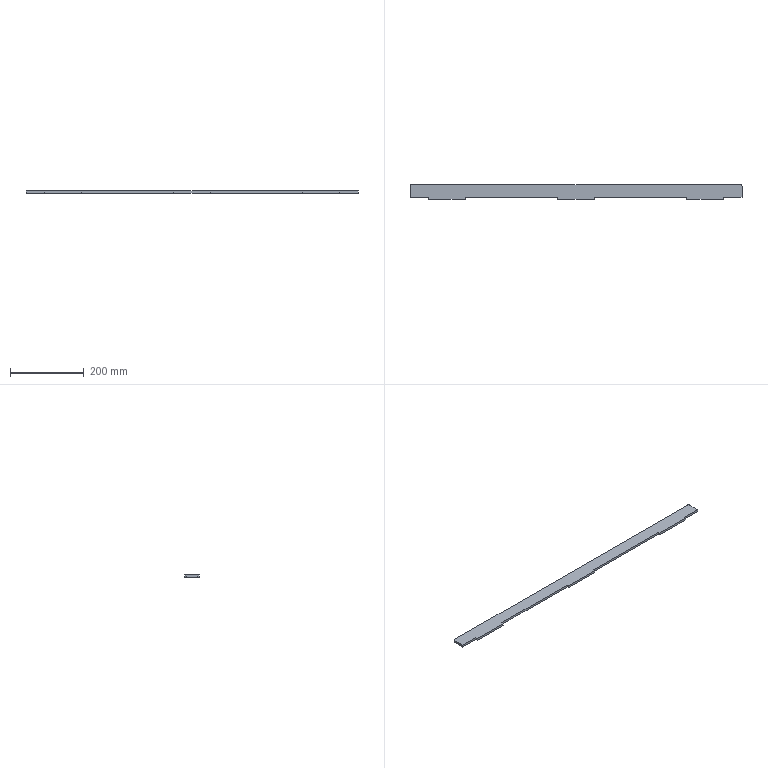Part | SolidWorks | features FlatPattern 1, SMBaseFlange 1, SheetMetal 1 | 1 solid | 20 faces | box 900 x 40.5 x 6 mm | volume 198836 mm3 | plane 18 | cylinder 2 | commonest cylinder face diameters 10 x2
STEP:
#1=CARTESIAN_POINT('',(439.219,-825.02,0.));
#2=VERTEX_POINT('',#1);
#3=CARTESIAN_POINT('',(489.219,-825.02,0.));
#4=VERTEX_POINT('',#3);
#5=CARTESIAN_POINT('',(489.219,-825.02,0.));
#6=DIRECTION('',(1.,0.,0.));
#7=VECTOR('',#6,1000.);
#8=LINE('',#5,#7);
#9=EDGE_CURVE('',#2,#4,#8,.T.);
#10=ORIENTED_EDGE('',*,*,#9,.T.);
#11=CARTESIAN_POINT('',(489.219,-825.02,6.));
#12=VERTEX_POINT('',#11);
#13=CARTESIAN_POINT('',(489.219,-825.02,6.));
#14=DIRECTION('',(0.,0.,-1.));
#15=VECTOR('',#14,1000.);
#16=LINE('',#13,#15);
#17=EDGE_CURVE('',#12,#4,#16,.T.);
#18=ORIENTED_EDGE('',*,*,#17,.F.);
#19=CARTESIAN_POINT('',(439.219,-825.02,6.));
#20=VERTEX_POINT('',#19);
#21=CARTESIAN_POINT('',(489.219,-825.02,6.));
#22=DIRECTION('',(1.,0.,0.));
#23=VECTOR('',#22,1000.);
#24=LINE('',#21,#23);
#25=EDGE_CURVE('',#20,#12,#24,.T.);
#26=ORIENTED_EDGE('',*,*,#25,.F.);
#27=CARTESIAN_POINT('',(439.219,-825.02,6.));
#28=DIRECTION('',(0.,0.,-1.));
#29=VECTOR('',#28,1000.);
#30=LINE('',#27,#29);
#31=EDGE_CURVE('',#20,#2,#30,.T.);
#32=ORIENTED_EDGE('',*,*,#31,.T.);
#33=EDGE_LOOP('',(#10,#18,#26,#32));
#34=FACE_OUTER_BOUND('',#33,.T.);
#35=CARTESIAN_POINT('',(489.219,-825.02,6.));
#36=DIRECTION('',(0.,1.,0.));
#37=DIRECTION('',(0.,0.,1.));
#38=AXIS2_PLACEMENT_3D('',#35,#36,#37);
#39=PLANE('',#38);
#40=ADVANCED_FACE('',(#34),#39,.F.);
#41=CARTESIAN_POINT('',(489.219,-795.02,0.));
#42=VERTEX_POINT('',#41);
#43=CARTESIAN_POINT('',(489.219,-825.02,0.));
#44=DIRECTION('',(0.,1.,0.));
#45=VECTOR('',#44,1000.);
#46=LINE('',#43,#45);
#47=EDGE_CURVE('',#4,#42,#46,.T.);
#48=ORIENTED_EDGE('',*,*,#47,.T.);
#49=CARTESIAN_POINT('',(489.219,-795.02,6.));
#50=VERTEX_POINT('',#49);
#51=CARTESIAN_POINT('',(489.219,-795.02,6.));
#52=DIRECTION('',(0.,0.,-1.));
#53=VECTOR('',#52,1000.);
#54=LINE('',#51,#53);
#55=EDGE_CURVE('',#50,#42,#54,.T.);
#56=ORIENTED_EDGE('',*,*,#55,.F.);
#57=CARTESIAN_POINT('',(489.219,-825.02,6.));
#58=DIRECTION('',(0.,1.,0.));
#59=VECTOR('',#58,1000.);
#60=LINE('',#57,#59);
#61=EDGE_CURVE('',#12,#50,#60,.T.);
#62=ORIENTED_EDGE('',*,*,#61,.F.);
#63=ORIENTED_EDGE('',*,*,#17,.T.);
#64=EDGE_LOOP('',(#48,#56,#62,#63));
#65=FACE_OUTER_BOUND('',#64,.T.);
#66=CARTESIAN_POINT('',(489.219,-825.02,6.));
#67=DIRECTION('',(-1.,0.,0.));
#68=DIRECTION('',(0.,0.,1.));
#69=AXIS2_PLACEMENT_3D('',#66,#67,#68);
#70=PLANE('',#69);
#71=ADVANCED_FACE('',(#65),#70,.F.);
#72=CARTESIAN_POINT('',(484.219,-790.02,0.));
#73=VERTEX_POINT('',#72);
#74=CARTESIAN_POINT('',(484.219,-795.02,0.));
#75=DIRECTION('',(0.,0.,1.));
#76=DIRECTION('',(1.,0.,0.));
#77=AXIS2_PLACEMENT_3D('',#74,#75,#76);
#78=CIRCLE('',#77,5.);
#79=EDGE_CURVE('',#42,#73,#78,.T.);
#80=ORIENTED_EDGE('',*,*,#79,.T.);
#81=CARTESIAN_POINT('',(484.219,-790.02,6.));
#82=VERTEX_POINT('',#81);
#83=CARTESIAN_POINT('',(484.219,-790.02,6.));
#84=DIRECTION('',(0.,0.,-1.));
#85=VECTOR('',#84,1000.);
#86=LINE('',#83,#85);
#87=EDGE_CURVE('',#82,#73,#86,.T.);
#88=ORIENTED_EDGE('',*,*,#87,.F.);
#89=CARTESIAN_POINT('',(484.219,-795.02,6.));
#90=DIRECTION('',(0.,0.,1.));
#91=DIRECTION('',(1.,0.,0.));
#92=AXIS2_PLACEMENT_3D('',#89,#90,#91);
#93=CIRCLE('',#92,5.);
#94=EDGE_CURVE('',#50,#82,#93,.T.);
#95=ORIENTED_EDGE('',*,*,#94,.F.);
#96=ORIENTED_EDGE('',*,*,#55,.T.);
#97=EDGE_LOOP('',(#80,#88,#95,#96));
#98=FACE_OUTER_BOUND('',#97,.T.);
#99=CARTESIAN_POINT('',(484.219,-795.02,6.));
#100=DIRECTION('',(0.,0.,-1.));
#101=DIRECTION('',(-1.,0.,0.));
#102=AXIS2_PLACEMENT_3D('',#99,#100,#101);
#103=CYLINDRICAL_SURFACE('',#102,5.);
#104=ADVANCED_FACE('',(#98),#103,.T.);
#105=CARTESIAN_POINT('',(-405.781,-790.02,0.));
#106=VERTEX_POINT('',#105);
#107=CARTESIAN_POINT('',(484.219,-790.02,0.));
#108=DIRECTION('',(-1.,0.,0.));
#109=VECTOR('',#108,1000.);
#110=LINE('',#107,#109);
#111=EDGE_CURVE('',#73,#106,#110,.T.);
#112=ORIENTED_EDGE('',*,*,#111,.T.);
#113=CARTESIAN_POINT('',(-405.781,-790.02,6.));
#114=VERTEX_POINT('',#113);
#115=CARTESIAN_POINT('',(-405.781,-790.02,6.));
#116=DIRECTION('',(0.,0.,-1.));
#117=VECTOR('',#116,1000.);
#118=LINE('',#115,#117);
#119=EDGE_CURVE('',#114,#106,#118,.T.);
#120=ORIENTED_EDGE('',*,*,#119,.F.);
#121=CARTESIAN_POINT('',(484.219,-790.02,6.));
#122=DIRECTION('',(-1.,0.,0.));
#123=VECTOR('',#122,1000.);
#124=LINE('',#121,#123);
#125=EDGE_CURVE('',#82,#114,#124,.T.);
#126=ORIENTED_EDGE('',*,*,#125,.F.);
#127=ORIENTED_EDGE('',*,*,#87,.T.);
#128=EDGE_LOOP('',(#112,#120,#126,#127));
#129=FACE_OUTER_BOUND('',#128,.T.);
#130=CARTESIAN_POINT('',(484.219,-790.02,6.));
#131=DIRECTION('',(0.,-1.,0.));
#132=DIRECTION('',(1.,0.,0.));
#133=AXIS2_PLACEMENT_3D('',#130,#131,#132);
#134=PLANE('',#133);
#135=ADVANCED_FACE('',(#129),#134,.F.);
#136=CARTESIAN_POINT('',(-410.781,-795.02,0.));
#137=VERTEX_POINT('',#136);
#138=CARTESIAN_POINT('',(-405.781,-795.02,0.));
#139=DIRECTION('',(0.,0.,1.));
#140=DIRECTION('',(1.,0.,0.));
#141=AXIS2_PLACEMENT_3D('',#138,#139,#140);
#142=CIRCLE('',#141,5.);
#143=EDGE_CURVE('',#106,#137,#142,.T.);
#144=ORIENTED_EDGE('',*,*,#143,.T.);
#145=CARTESIAN_POINT('',(-410.781,-795.02,6.));
#146=VERTEX_POINT('',#145);
#147=CARTESIAN_POINT('',(-410.781,-795.02,6.));
#148=DIRECTION('',(0.,0.,-1.));
#149=VECTOR('',#148,1000.);
#150=LINE('',#147,#149);
#151=EDGE_CURVE('',#146,#137,#150,.T.);
#152=ORIENTED_EDGE('',*,*,#151,.F.);
#153=CARTESIAN_POINT('',(-405.781,-795.02,6.));
#154=DIRECTION('',(0.,0.,1.));
#155=DIRECTION('',(1.,0.,0.));
#156=AXIS2_PLACEMENT_3D('',#153,#154,#155);
#157=CIRCLE('',#156,5.);
#158=EDGE_CURVE('',#114,#146,#157,.T.);
#159=ORIENTED_EDGE('',*,*,#158,.F.);
#160=ORIENTED_EDGE('',*,*,#119,.T.);
#161=EDGE_LOOP('',(#144,#152,#159,#160));
#162=FACE_OUTER_BOUND('',#161,.T.);
#163=CARTESIAN_POINT('',(-405.781,-795.02,6.));
#164=DIRECTION('',(0.,0.,-1.));
#165=DIRECTION('',(-1.,0.,0.));
#166=AXIS2_PLACEMENT_3D('',#163,#164,#165);
#167=CYLINDRICAL_SURFACE('',#166,5.);
#168=ADVANCED_FACE('',(#162),#167,.T.);
#169=CARTESIAN_POINT('',(-410.781,-825.02,0.));
#170=VERTEX_POINT('',#169);
#171=CARTESIAN_POINT('',(-410.781,-825.02,0.));
#172=DIRECTION('',(0.,-1.,0.));
#173=VECTOR('',#172,1000.);
#174=LINE('',#171,#173);
#175=EDGE_CURVE('',#137,#170,#174,.T.);
#176=ORIENTED_EDGE('',*,*,#175,.T.);
#177=CARTESIAN_POINT('',(-410.781,-825.02,6.));
#178=VERTEX_POINT('',#177);
#179=CARTESIAN_POINT('',(-410.781,-825.02,6.));
#180=DIRECTION('',(0.,0.,-1.));
#181=VECTOR('',#180,1000.);
#182=LINE('',#179,#181);
#183=EDGE_CURVE('',#178,#170,#182,.T.);
#184=ORIENTED_EDGE('',*,*,#183,.F.);
#185=CARTESIAN_POINT('',(-410.781,-825.02,6.));
#186=DIRECTION('',(0.,-1.,0.));
#187=VECTOR('',#186,1000.);
#188=LINE('',#185,#187);
#189=EDGE_CURVE('',#146,#178,#188,.T.);
#190=ORIENTED_EDGE('',*,*,#189,.F.);
#191=ORIENTED_EDGE('',*,*,#151,.T.);
#192=EDGE_LOOP('',(#176,#184,#190,#191));
#193=FACE_OUTER_BOUND('',#192,.T.);
#194=CARTESIAN_POINT('',(-410.781,-825.02,6.));
#195=DIRECTION('',(1.,0.,0.));
#196=DIRECTION('',(0.,1.,0.));
#197=AXIS2_PLACEMENT_3D('',#194,#195,#196);
#198=PLANE('',#197);
#199=ADVANCED_FACE('',(#193),#198,.F.);
#200=CARTESIAN_POINT('',(-360.781,-825.02,0.));
#201=VERTEX_POINT('',#200);
#202=CARTESIAN_POINT('',(-360.781,-825.02,0.));
#203=DIRECTION('',(1.,0.,0.));
#204=VECTOR('',#203,1000.);
#205=LINE('',#202,#204);
#206=EDGE_CURVE('',#170,#201,#205,.T.);
#207=ORIENTED_EDGE('',*,*,#206,.T.);
#208=CARTESIAN_POINT('',(-360.781,-825.02,6.));
#209=VERTEX_POINT('',#208);
#210=CARTESIAN_POINT('',(-360.781,-825.02,6.));
#211=DIRECTION('',(0.,0.,-1.));
#212=VECTOR('',#211,1000.);
#213=LINE('',#210,#212);
#214=EDGE_CURVE('',#209,#201,#213,.T.);
#215=ORIENTED_EDGE('',*,*,#214,.F.);
#216=CARTESIAN_POINT('',(-360.781,-825.02,6.));
#217=DIRECTION('',(1.,0.,0.));
#218=VECTOR('',#217,1000.);
#219=LINE('',#216,#218);
#220=EDGE_CURVE('',#178,#209,#219,.T.);
#221=ORIENTED_EDGE('',*,*,#220,.F.);
#222=ORIENTED_EDGE('',*,*,#183,.T.);
#223=EDGE_LOOP('',(#207,#215,#221,#222));
#224=FACE_OUTER_BOUND('',#223,.T.);
#225=CARTESIAN_POINT('',(-360.781,-825.02,6.));
#226=DIRECTION('',(0.,1.,0.));
#227=DIRECTION('',(-1.,0.,0.));
#228=AXIS2_PLACEMENT_3D('',#225,#226,#227);
#229=PLANE('',#228);
#230=ADVANCED_FACE('',(#224),#229,.F.);
#231=CARTESIAN_POINT('',(-360.781,-830.52,0.));
#232=VERTEX_POINT('',#231);
#233=CARTESIAN_POINT('',(-360.781,-830.52,0.));
#234=DIRECTION('',(0.,-1.,0.));
#235=VECTOR('',#234,1000.);
#236=LINE('',#233,#235);
#237=EDGE_CURVE('',#201,#232,#236,.T.);
#238=ORIENTED_EDGE('',*,*,#237,.T.);
#239=CARTESIAN_POINT('',(-360.781,-830.52,6.));
#240=VERTEX_POINT('',#239);
#241=CARTESIAN_POINT('',(-360.781,-830.52,6.));
#242=DIRECTION('',(0.,0.,-1.));
#243=VECTOR('',#242,1000.);
#244=LINE('',#241,#243);
#245=EDGE_CURVE('',#240,#232,#244,.T.);
#246=ORIENTED_EDGE('',*,*,#245,.F.);
#247=CARTESIAN_POINT('',(-360.781,-830.52,6.));
#248=DIRECTION('',(0.,-1.,0.));
#249=VECTOR('',#248,1000.);
#250=LINE('',#247,#249);
#251=EDGE_CURVE('',#209,#240,#250,.T.);
#252=ORIENTED_EDGE('',*,*,#251,.F.);
#253=ORIENTED_EDGE('',*,*,#214,.T.);
#254=EDGE_LOOP('',(#238,#246,#252,#253));
#255=FACE_OUTER_BOUND('',#254,.T.);
#256=CARTESIAN_POINT('',(-360.781,-830.52,6.));
#257=DIRECTION('',(1.,0.,0.));
#258=DIRECTION('',(0.,0.,-1.));
#259=AXIS2_PLACEMENT_3D('',#256,#257,#258);
#260=PLANE('',#259);
#261=ADVANCED_FACE('',(#255),#260,.F.);
#262=CARTESIAN_POINT('',(-260.781,-830.52,0.));
#263=VERTEX_POINT('',#262);
#264=CARTESIAN_POINT('',(-260.781,-830.52,0.));
#265=DIRECTION('',(1.,0.,0.));
#266=VECTOR('',#265,1000.);
#267=LINE('',#264,#266);
#268=EDGE_CURVE('',#232,#263,#267,.T.);
#269=ORIENTED_EDGE('',*,*,#268,.T.);
#270=CARTESIAN_POINT('',(-260.781,-830.52,6.));
#271=VERTEX_POINT('',#270);
#272=CARTESIAN_POINT('',(-260.781,-830.52,6.));
#273=DIRECTION('',(0.,0.,-1.));
#274=VECTOR('',#273,1000.);
#275=LINE('',#272,#274);
#276=EDGE_CURVE('',#271,#263,#275,.T.);
#277=ORIENTED_EDGE('',*,*,#276,.F.);
#278=CARTESIAN_POINT('',(-260.781,-830.52,6.));
#279=DIRECTION('',(1.,0.,0.));
#280=VECTOR('',#279,1000.);
#281=LINE('',#278,#280);
#282=EDGE_CURVE('',#240,#271,#281,.T.);
#283=ORIENTED_EDGE('',*,*,#282,.F.);
#284=ORIENTED_EDGE('',*,*,#245,.T.);
#285=EDGE_LOOP('',(#269,#277,#283,#284));
#286=FACE_OUTER_BOUND('',#285,.T.);
#287=CARTESIAN_POINT('',(-260.781,-830.52,6.));
#288=DIRECTION('',(0.,1.,0.));
#289=DIRECTION('',(0.,0.,1.));
#290=AXIS2_PLACEMENT_3D('',#287,#288,#289);
#291=PLANE('',#290);
#292=ADVANCED_FACE('',(#286),#291,.F.);
#293=CARTESIAN_POINT('',(-260.781,-825.02,0.));
#294=VERTEX_POINT('',#293);
#295=CARTESIAN_POINT('',(-260.781,-825.02,0.));
#296=DIRECTION('',(0.,1.,0.));
#297=VECTOR('',#296,1000.);
#298=LINE('',#295,#297);
#299=EDGE_CURVE('',#263,#294,#298,.T.);
#300=ORIENTED_EDGE('',*,*,#299,.T.);
#301=CARTESIAN_POINT('',(-260.781,-825.02,6.));
#302=VERTEX_POINT('',#301);
#303=CARTESIAN_POINT('',(-260.781,-825.02,6.));
#304=DIRECTION('',(0.,0.,-1.));
#305=VECTOR('',#304,1000.);
#306=LINE('',#303,#305);
#307=EDGE_CURVE('',#302,#294,#306,.T.);
#308=ORIENTED_EDGE('',*,*,#307,.F.);
#309=CARTESIAN_POINT('',(-260.781,-825.02,6.));
#310=DIRECTION('',(0.,1.,0.));
#311=VECTOR('',#310,1000.);
#312=LINE('',#309,#311);
#313=EDGE_CURVE('',#271,#302,#312,.T.);
#314=ORIENTED_EDGE('',*,*,#313,.F.);
#315=ORIENTED_EDGE('',*,*,#276,.T.);
#316=EDGE_LOOP('',(#300,#308,#314,#315));
#317=FACE_OUTER_BOUND('',#316,.T.);
#318=CARTESIAN_POINT('',(-260.781,-825.02,6.));
#319=DIRECTION('',(-1.,0.,0.));
#320=DIRECTION('',(0.,0.,1.));
#321=AXIS2_PLACEMENT_3D('',#318,#319,#320);
#322=PLANE('',#321);
#323=ADVANCED_FACE('',(#317),#322,.F.);
#324=CARTESIAN_POINT('',(-10.781,-825.02,0.));
#325=VERTEX_POINT('',#324);
#326=CARTESIAN_POINT('',(-10.781,-825.02,0.));
#327=DIRECTION('',(1.,0.,0.));
#328=VECTOR('',#327,1000.);
#329=LINE('',#326,#328);
#330=EDGE_CURVE('',#294,#325,#329,.T.);
#331=ORIENTED_EDGE('',*,*,#330,.T.);
#332=CARTESIAN_POINT('',(-10.781,-825.02,6.));
#333=VERTEX_POINT('',#332);
#334=CARTESIAN_POINT('',(-10.781,-825.02,6.));
#335=DIRECTION('',(0.,0.,-1.));
#336=VECTOR('',#335,1000.);
#337=LINE('',#334,#336);
#338=EDGE_CURVE('',#333,#325,#337,.T.);
#339=ORIENTED_EDGE('',*,*,#338,.F.);
#340=CARTESIAN_POINT('',(-10.781,-825.02,6.));
#341=DIRECTION('',(1.,0.,0.));
#342=VECTOR('',#341,1000.);
#343=LINE('',#340,#342);
#344=EDGE_CURVE('',#302,#333,#343,.T.);
#345=ORIENTED_EDGE('',*,*,#344,.F.);
#346=ORIENTED_EDGE('',*,*,#307,.T.);
#347=EDGE_LOOP('',(#331,#339,#345,#346));
#348=FACE_OUTER_BOUND('',#347,.T.);
#349=CARTESIAN_POINT('',(-10.781,-825.02,6.));
#350=DIRECTION('',(0.,1.,0.));
#351=DIRECTION('',(-1.,0.,0.));
#352=AXIS2_PLACEMENT_3D('',#349,#350,#351);
#353=PLANE('',#352);
#354=ADVANCED_FACE('',(#348),#353,.F.);
#355=CARTESIAN_POINT('',(-10.781,-830.52,0.));
#356=VERTEX_POINT('',#355);
#357=CARTESIAN_POINT('',(-10.781,-830.52,0.));
#358=DIRECTION('',(0.,-1.,0.));
#359=VECTOR('',#358,1000.);
#360=LINE('',#357,#359);
#361=EDGE_CURVE('',#325,#356,#360,.T.);
#362=ORIENTED_EDGE('',*,*,#361,.T.);
#363=CARTESIAN_POINT('',(-10.781,-830.52,6.));
#364=VERTEX_POINT('',#363);
#365=CARTESIAN_POINT('',(-10.781,-830.52,6.));
#366=DIRECTION('',(0.,0.,-1.));
#367=VECTOR('',#366,1000.);
#368=LINE('',#365,#367);
#369=EDGE_CURVE('',#364,#356,#368,.T.);
#370=ORIENTED_EDGE('',*,*,#369,.F.);
#371=CARTESIAN_POINT('',(-10.781,-830.52,6.));
#372=DIRECTION('',(0.,-1.,0.));
#373=VECTOR('',#372,1000.);
#374=LINE('',#371,#373);
#375=EDGE_CURVE('',#333,#364,#374,.T.);
#376=ORIENTED_EDGE('',*,*,#375,.F.);
#377=ORIENTED_EDGE('',*,*,#338,.T.);
#378=EDGE_LOOP('',(#362,#370,#376,#377));
#379=FACE_OUTER_BOUND('',#378,.T.);
#380=CARTESIAN_POINT('',(-10.781,-830.52,6.));
#381=DIRECTION('',(1.,0.,0.));
#382=DIRECTION('',(0.,0.,-1.));
#383=AXIS2_PLACEMENT_3D('',#380,#381,#382);
#384=PLANE('',#383);
#385=ADVANCED_FACE('',(#379),#384,.F.);
#386=CARTESIAN_POINT('',(89.219,-830.52,0.));
#387=VERTEX_POINT('',#386);
#388=CARTESIAN_POINT('',(89.219,-830.52,0.));
#389=DIRECTION('',(1.,0.,0.));
#390=VECTOR('',#389,1000.);
#391=LINE('',#388,#390);
#392=EDGE_CURVE('',#356,#387,#391,.T.);
#393=ORIENTED_EDGE('',*,*,#392,.T.);
#394=CARTESIAN_POINT('',(89.219,-830.52,6.));
#395=VERTEX_POINT('',#394);
#396=CARTESIAN_POINT('',(89.219,-830.52,6.));
#397=DIRECTION('',(0.,0.,-1.));
#398=VECTOR('',#397,1000.);
#399=LINE('',#396,#398);
#400=EDGE_CURVE('',#395,#387,#399,.T.);
#401=ORIENTED_EDGE('',*,*,#400,.F.);
#402=CARTESIAN_POINT('',(89.219,-830.52,6.));
#403=DIRECTION('',(1.,0.,0.));
#404=VECTOR('',#403,1000.);
#405=LINE('',#402,#404);
#406=EDGE_CURVE('',#364,#395,#405,.T.);
#407=ORIENTED_EDGE('',*,*,#406,.F.);
#408=ORIENTED_EDGE('',*,*,#369,.T.);
#409=EDGE_LOOP('',(#393,#401,#407,#408));
#410=FACE_OUTER_BOUND('',#409,.T.);
#411=CARTESIAN_POINT('',(89.219,-830.52,6.));
#412=DIRECTION('',(0.,1.,0.));
#413=DIRECTION('',(0.,0.,1.));
#414=AXIS2_PLACEMENT_3D('',#411,#412,#413);
#415=PLANE('',#414);
#416=ADVANCED_FACE('',(#410),#415,.F.);
#417=CARTESIAN_POINT('',(89.219,-825.02,0.));
#418=VERTEX_POINT('',#417);
#419=CARTESIAN_POINT('',(89.219,-825.02,0.));
#420=DIRECTION('',(0.,1.,0.));
#421=VECTOR('',#420,1000.);
#422=LINE('',#419,#421);
#423=EDGE_CURVE('',#387,#418,#422,.T.);
#424=ORIENTED_EDGE('',*,*,#423,.T.);
#425=CARTESIAN_POINT('',(89.219,-825.02,6.));
#426=VERTEX_POINT('',#425);
#427=CARTESIAN_POINT('',(89.219,-825.02,6.));
#428=DIRECTION('',(0.,0.,-1.));
#429=VECTOR('',#428,1000.);
#430=LINE('',#427,#429);
#431=EDGE_CURVE('',#426,#418,#430,.T.);
#432=ORIENTED_EDGE('',*,*,#431,.F.);
#433=CARTESIAN_POINT('',(89.219,-825.02,6.));
#434=DIRECTION('',(0.,1.,0.));
#435=VECTOR('',#434,1000.);
#436=LINE('',#433,#435);
#437=EDGE_CURVE('',#395,#426,#436,.T.);
#438=ORIENTED_EDGE('',*,*,#437,.F.);
#439=ORIENTED_EDGE('',*,*,#400,.T.);
#440=EDGE_LOOP('',(#424,#432,#438,#439));
#441=FACE_OUTER_BOUND('',#440,.T.);
#442=CARTESIAN_POINT('',(89.219,-825.02,6.));
#443=DIRECTION('',(-1.,0.,0.));
#444=DIRECTION('',(0.,0.,1.));
#445=AXIS2_PLACEMENT_3D('',#442,#443,#444);
#446=PLANE('',#445);
#447=ADVANCED_FACE('',(#441),#446,.F.);
#448=CARTESIAN_POINT('',(339.219,-825.02,0.));
#449=VERTEX_POINT('',#448);
#450=CARTESIAN_POINT('',(339.219,-825.02,0.));
#451=DIRECTION('',(1.,0.,0.));
#452=VECTOR('',#451,1000.);
#453=LINE('',#450,#452);
#454=EDGE_CURVE('',#418,#449,#453,.T.);
#455=ORIENTED_EDGE('',*,*,#454,.T.);
#456=CARTESIAN_POINT('',(339.219,-825.02,6.));
#457=VERTEX_POINT('',#456);
#458=CARTESIAN_POINT('',(339.219,-825.02,6.));
#459=DIRECTION('',(0.,0.,-1.));
#460=VECTOR('',#459,1000.);
#461=LINE('',#458,#460);
#462=EDGE_CURVE('',#457,#449,#461,.T.);
#463=ORIENTED_EDGE('',*,*,#462,.F.);
#464=CARTESIAN_POINT('',(339.219,-825.02,6.));
#465=DIRECTION('',(1.,0.,0.));
#466=VECTOR('',#465,1000.);
#467=LINE('',#464,#466);
#468=EDGE_CURVE('',#426,#457,#467,.T.);
#469=ORIENTED_EDGE('',*,*,#468,.F.);
#470=ORIENTED_EDGE('',*,*,#431,.T.);
#471=EDGE_LOOP('',(#455,#463,#469,#470));
#472=FACE_OUTER_BOUND('',#471,.T.);
#473=CARTESIAN_POINT('',(339.219,-825.02,6.));
#474=DIRECTION('',(0.,1.,0.));
#475=DIRECTION('',(-1.,0.,0.));
#476=AXIS2_PLACEMENT_3D('',#473,#474,#475);
#477=PLANE('',#476);
#478=ADVANCED_FACE('',(#472),#477,.F.);
#479=CARTESIAN_POINT('',(339.219,-830.52,0.));
#480=VERTEX_POINT('',#479);
#481=CARTESIAN_POINT('',(339.219,-830.52,0.));
#482=DIRECTION('',(0.,-1.,0.));
#483=VECTOR('',#482,1000.);
#484=LINE('',#481,#483);
#485=EDGE_CURVE('',#449,#480,#484,.T.);
#486=ORIENTED_EDGE('',*,*,#485,.T.);
#487=CARTESIAN_POINT('',(339.219,-830.52,6.));
#488=VERTEX_POINT('',#487);
#489=CARTESIAN_POINT('',(339.219,-830.52,6.));
#490=DIRECTION('',(0.,0.,-1.));
#491=VECTOR('',#490,1000.);
#492=LINE('',#489,#491);
#493=EDGE_CURVE('',#488,#480,#492,.T.);
#494=ORIENTED_EDGE('',*,*,#493,.F.);
#495=CARTESIAN_POINT('',(339.219,-830.52,6.));
#496=DIRECTION('',(0.,-1.,0.));
#497=VECTOR('',#496,1000.);
#498=LINE('',#495,#497);
#499=EDGE_CURVE('',#457,#488,#498,.T.);
#500=ORIENTED_EDGE('',*,*,#499,.F.);
#501=ORIENTED_EDGE('',*,*,#462,.T.);
#502=EDGE_LOOP('',(#486,#494,#500,#501));
#503=FACE_OUTER_BOUND('',#502,.T.);
#504=CARTESIAN_POINT('',(339.219,-830.52,6.));
#505=DIRECTION('',(1.,0.,0.));
#506=DIRECTION('',(0.,0.,-1.));
#507=AXIS2_PLACEMENT_3D('',#504,#505,#506);
#508=PLANE('',#507);
#509=ADVANCED_FACE('',(#503),#508,.F.);
#510=CARTESIAN_POINT('',(439.219,-830.52,0.));
#511=VERTEX_POINT('',#510);
#512=CARTESIAN_POINT('',(439.219,-830.52,0.));
#513=DIRECTION('',(1.,0.,0.));
#514=VECTOR('',#513,1000.);
#515=LINE('',#512,#514);
#516=EDGE_CURVE('',#480,#511,#515,.T.);
#517=ORIENTED_EDGE('',*,*,#516,.T.);
#518=CARTESIAN_POINT('',(439.219,-830.52,6.));
#519=VERTEX_POINT('',#518);
#520=CARTESIAN_POINT('',(439.219,-830.52,6.));
#521=DIRECTION('',(0.,0.,-1.));
#522=VECTOR('',#521,1000.);
#523=LINE('',#520,#522);
#524=EDGE_CURVE('',#519,#511,#523,.T.);
#525=ORIENTED_EDGE('',*,*,#524,.F.);
#526=CARTESIAN_POINT('',(439.219,-830.52,6.));
#527=DIRECTION('',(1.,0.,0.));
#528=VECTOR('',#527,1000.);
#529=LINE('',#526,#528);
#530=EDGE_CURVE('',#488,#519,#529,.T.);
#531=ORIENTED_EDGE('',*,*,#530,.F.);
#532=ORIENTED_EDGE('',*,*,#493,.T.);
#533=EDGE_LOOP('',(#517,#525,#531,#532));
#534=FACE_OUTER_BOUND('',#533,.T.);
#535=CARTESIAN_POINT('',(439.219,-830.52,6.));
#536=DIRECTION('',(0.,1.,0.));
#537=DIRECTION('',(0.,0.,1.));
#538=AXIS2_PLACEMENT_3D('',#535,#536,#537);
#539=PLANE('',#538);
#540=ADVANCED_FACE('',(#534),#539,.F.);
#541=CARTESIAN_POINT('',(439.219,-825.02,0.));
#542=DIRECTION('',(0.,1.,0.));
#543=VECTOR('',#542,1000.);
#544=LINE('',#541,#543);
#545=EDGE_CURVE('',#511,#2,#544,.T.);
#546=ORIENTED_EDGE('',*,*,#545,.T.);
#547=ORIENTED_EDGE('',*,*,#31,.F.);
#548=CARTESIAN_POINT('',(439.219,-825.02,6.));
#549=DIRECTION('',(0.,1.,0.));
#550=VECTOR('',#549,1000.);
#551=LINE('',#548,#550);
#552=EDGE_CURVE('',#519,#20,#551,.T.);
#553=ORIENTED_EDGE('',*,*,#552,.F.);
#554=ORIENTED_EDGE('',*,*,#524,.T.);
#555=EDGE_LOOP('',(#546,#547,#553,#554));
#556=FACE_OUTER_BOUND('',#555,.T.);
#557=CARTESIAN_POINT('',(439.219,-825.02,6.));
#558=DIRECTION('',(-1.,0.,0.));
#559=DIRECTION('',(0.,0.,1.));
#560=AXIS2_PLACEMENT_3D('',#557,#558,#559);
#561=PLANE('',#560);
#562=ADVANCED_FACE('',(#556),#561,.F.);
#563=ORIENTED_EDGE('',*,*,#25,.T.);
#564=ORIENTED_EDGE('',*,*,#61,.T.);
#565=ORIENTED_EDGE('',*,*,#94,.T.);
#566=ORIENTED_EDGE('',*,*,#125,.T.);
#567=ORIENTED_EDGE('',*,*,#158,.T.);
#568=ORIENTED_EDGE('',*,*,#189,.T.);
#569=ORIENTED_EDGE('',*,*,#220,.T.);
#570=ORIENTED_EDGE('',*,*,#251,.T.);
#571=ORIENTED_EDGE('',*,*,#282,.T.);
#572=ORIENTED_EDGE('',*,*,#313,.T.);
#573=ORIENTED_EDGE('',*,*,#344,.T.);
#574=ORIENTED_EDGE('',*,*,#375,.T.);
#575=ORIENTED_EDGE('',*,*,#406,.T.);
#576=ORIENTED_EDGE('',*,*,#437,.T.);
#577=ORIENTED_EDGE('',*,*,#468,.T.);
#578=ORIENTED_EDGE('',*,*,#499,.T.);
#579=ORIENTED_EDGE('',*,*,#530,.T.);
#580=ORIENTED_EDGE('',*,*,#552,.T.);
#581=EDGE_LOOP('',(#563,#564,#565,#566,#567,#568,#569,#570,#571,#572,#573,#574,#575,#576,#577,#578,#579,#580));
#582=FACE_OUTER_BOUND('',#581,.T.);
#583=CARTESIAN_POINT('',(-405.781,-795.02,6.));
#584=DIRECTION('',(0.,0.,1.));
#585=DIRECTION('',(1.,0.,0.));
#586=AXIS2_PLACEMENT_3D('',#583,#584,#585);
#587=PLANE('',#586);
#588=ADVANCED_FACE('',(#582),#587,.T.);
#589=ORIENTED_EDGE('',*,*,#9,.F.);
#590=ORIENTED_EDGE('',*,*,#545,.F.);
#591=ORIENTED_EDGE('',*,*,#516,.F.);
#592=ORIENTED_EDGE('',*,*,#485,.F.);
#593=ORIENTED_EDGE('',*,*,#454,.F.);
#594=ORIENTED_EDGE('',*,*,#423,.F.);
#595=ORIENTED_EDGE('',*,*,#392,.F.);
#596=ORIENTED_EDGE('',*,*,#361,.F.);
#597=ORIENTED_EDGE('',*,*,#330,.F.);
#598=ORIENTED_EDGE('',*,*,#299,.F.);
#599=ORIENTED_EDGE('',*,*,#268,.F.);
#600=ORIENTED_EDGE('',*,*,#237,.F.);
#601=ORIENTED_EDGE('',*,*,#206,.F.);
#602=ORIENTED_EDGE('',*,*,#175,.F.);
#603=ORIENTED_EDGE('',*,*,#143,.F.);
#604=ORIENTED_EDGE('',*,*,#111,.F.);
#605=ORIENTED_EDGE('',*,*,#79,.F.);
#606=ORIENTED_EDGE('',*,*,#47,.F.);
#607=EDGE_LOOP('',(#589,#590,#591,#592,#593,#594,#595,#596,#597,#598,#599,#600,#601,#602,#603,#604,#605,#606));
#608=FACE_OUTER_BOUND('',#607,.T.);
#609=CARTESIAN_POINT('',(-405.781,-795.02,0.));
#610=DIRECTION('',(0.,0.,1.));
#611=DIRECTION('',(1.,0.,0.));
#612=AXIS2_PLACEMENT_3D('',#609,#610,#611);
#613=PLANE('',#612);
#614=ADVANCED_FACE('',(#608),#613,.F.);
#615=CLOSED_SHELL('',(#40,#71,#104,#135,#168,#199,#230,#261,#292,#323,#354,#385,#416,#447,#478,#509,#540,#562,#588,#614));
#616=MANIFOLD_SOLID_BREP('',#615);
#617=CARTESIAN_POINT('',(0.,0.,0.));
#618=DIRECTION('',(0.,0.,1.));
#619=DIRECTION('',(1.,0.,0.));
#620=AXIS2_PLACEMENT_3D('',#617,#618,#619);
#621=(LENGTH_UNIT()NAMED_UNIT(*)SI_UNIT(.MILLI.,.METRE.));
#622=UNCERTAINTY_MEASURE_WITH_UNIT(LENGTH_MEASURE(0.00001),#621,'','');
#623=(NAMED_UNIT(*)PLANE_ANGLE_UNIT()SI_UNIT($,.RADIAN.));
#624=(NAMED_UNIT(*)SI_UNIT($,.STERADIAN.)SOLID_ANGLE_UNIT());
#625=(GEOMETRIC_REPRESENTATION_CONTEXT(3)GLOBAL_UNCERTAINTY_ASSIGNED_CONTEXT((#622))GLOBAL_UNIT_ASSIGNED_CONTEXT((#621,#623,#624))REPRESENTATION_CONTEXT('',''));
#626=ADVANCED_BREP_SHAPE_REPRESENTATION('',(#616,#620),#625);